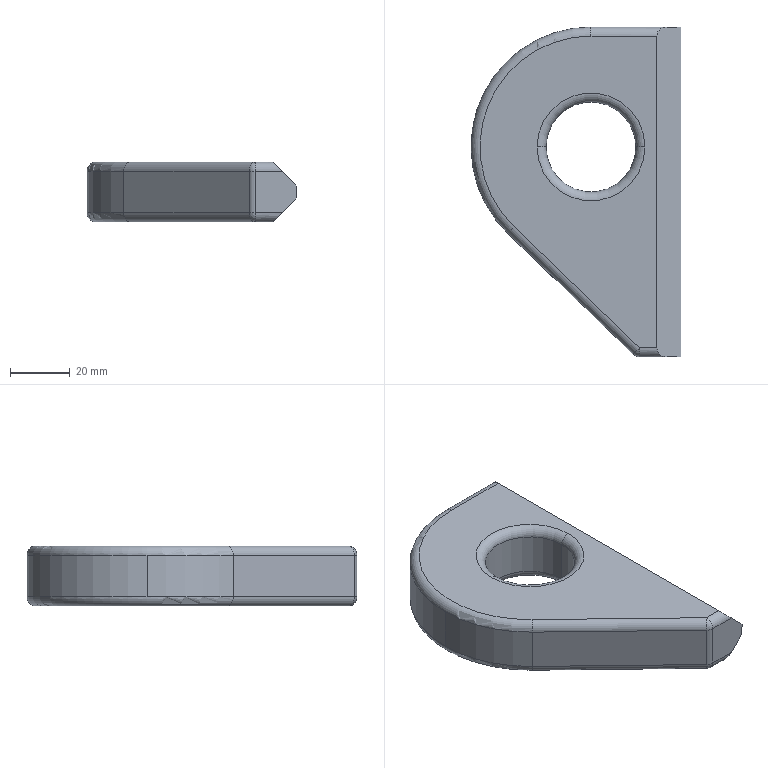Part | SolidWorks | features Fillet 3, Extrusion 1, ICE 1 | 1 solid | 27 faces | box 70 x 110 x 20 mm | volume 94979 mm3 | cylinder 11 | plane 8 | torus 6 | sphere 2 | commonest cylinder face diameters 6 x7 30 x2 80 x2
STEP:
#1=CARTESIAN_POINT('',(-15.,0.,3.));
#2=VERTEX_POINT('',#1);
#3=CARTESIAN_POINT('',(15.,0.,3.));
#4=VERTEX_POINT('',#3);
#5=CARTESIAN_POINT('',(0.,0.,3.));
#6=DIRECTION('',(0.,0.,-1.));
#7=DIRECTION('',(1.,0.,0.));
#8=AXIS2_PLACEMENT_3D('',#5,#6,#7);
#9=CIRCLE('',#8,15.);
#10=EDGE_CURVE('',#2,#4,#9,.T.);
#11=ORIENTED_EDGE('',*,*,#10,.F.);
#12=CARTESIAN_POINT('',(-18.,0.,0.));
#13=VERTEX_POINT('',#12);
#14=CARTESIAN_POINT('',(-18.,0.,3.));
#15=DIRECTION('',(0.,1.,0.));
#16=DIRECTION('',(0.,0.,1.));
#17=AXIS2_PLACEMENT_3D('',#14,#15,#16);
#18=CIRCLE('',#17,3.);
#19=EDGE_CURVE('',#2,#13,#18,.T.);
#20=ORIENTED_EDGE('',*,*,#19,.T.);
#21=CARTESIAN_POINT('',(18.,0.,0.));
#22=VERTEX_POINT('',#21);
#23=CARTESIAN_POINT('',(0.,0.,0.));
#24=DIRECTION('',(0.,0.,1.));
#25=DIRECTION('',(1.,0.,0.));
#26=AXIS2_PLACEMENT_3D('',#23,#24,#25);
#27=CIRCLE('',#26,18.);
#28=EDGE_CURVE('',#22,#13,#27,.T.);
#29=ORIENTED_EDGE('',*,*,#28,.F.);
#30=CARTESIAN_POINT('',(18.,0.,3.));
#31=DIRECTION('',(0.,-1.,0.));
#32=DIRECTION('',(0.,0.,-1.));
#33=AXIS2_PLACEMENT_3D('',#30,#31,#32);
#34=CIRCLE('',#33,3.);
#35=EDGE_CURVE('',#4,#22,#34,.T.);
#36=ORIENTED_EDGE('',*,*,#35,.F.);
#37=EDGE_LOOP('',(#11,#20,#29,#36));
#38=FACE_OUTER_BOUND('',#37,.T.);
#39=CARTESIAN_POINT('',(0.,0.,3.));
#40=DIRECTION('',(0.,0.,1.));
#41=DIRECTION('',(1.,0.,0.));
#42=AXIS2_PLACEMENT_3D('',#39,#40,#41);
#43=TOROIDAL_SURFACE('',#42,18.,3.);
#44=ADVANCED_FACE('',(#38),#43,.T.);
#45=CARTESIAN_POINT('',(-18.,0.,20.));
#46=VERTEX_POINT('',#45);
#47=CARTESIAN_POINT('',(18.,0.,20.));
#48=VERTEX_POINT('',#47);
#49=CARTESIAN_POINT('',(0.,0.,20.));
#50=DIRECTION('',(0.,0.,-1.));
#51=DIRECTION('',(1.,0.,0.));
#52=AXIS2_PLACEMENT_3D('',#49,#50,#51);
#53=CIRCLE('',#52,18.);
#54=EDGE_CURVE('',#46,#48,#53,.T.);
#55=ORIENTED_EDGE('',*,*,#54,.F.);
#56=CARTESIAN_POINT('',(-15.,0.,17.));
#57=VERTEX_POINT('',#56);
#58=CARTESIAN_POINT('',(-18.,0.,17.));
#59=DIRECTION('',(0.,1.,0.));
#60=DIRECTION('',(0.,0.,1.));
#61=AXIS2_PLACEMENT_3D('',#58,#59,#60);
#62=CIRCLE('',#61,3.);
#63=EDGE_CURVE('',#46,#57,#62,.T.);
#64=ORIENTED_EDGE('',*,*,#63,.T.);
#65=CARTESIAN_POINT('',(15.,0.,17.));
#66=VERTEX_POINT('',#65);
#67=CARTESIAN_POINT('',(0.,0.,17.));
#68=DIRECTION('',(0.,0.,1.));
#69=DIRECTION('',(1.,0.,0.));
#70=AXIS2_PLACEMENT_3D('',#67,#68,#69);
#71=CIRCLE('',#70,15.);
#72=EDGE_CURVE('',#66,#57,#71,.T.);
#73=ORIENTED_EDGE('',*,*,#72,.F.);
#74=CARTESIAN_POINT('',(18.,0.,17.));
#75=DIRECTION('',(0.,-1.,0.));
#76=DIRECTION('',(0.,0.,-1.));
#77=AXIS2_PLACEMENT_3D('',#74,#75,#76);
#78=CIRCLE('',#77,3.);
#79=EDGE_CURVE('',#48,#66,#78,.T.);
#80=ORIENTED_EDGE('',*,*,#79,.F.);
#81=EDGE_LOOP('',(#55,#64,#73,#80));
#82=FACE_OUTER_BOUND('',#81,.T.);
#83=CARTESIAN_POINT('',(0.,0.,17.));
#84=DIRECTION('',(0.,0.,1.));
#85=DIRECTION('',(1.,0.,0.));
#86=AXIS2_PLACEMENT_3D('',#83,#84,#85);
#87=TOROIDAL_SURFACE('',#86,18.,3.);
#88=ADVANCED_FACE('',(#82),#87,.T.);
#89=CARTESIAN_POINT('',(0.,0.,17.));
#90=DIRECTION('',(0.,0.,1.));
#91=DIRECTION('',(1.,0.,0.));
#92=AXIS2_PLACEMENT_3D('',#89,#90,#91);
#93=CIRCLE('',#92,15.);
#94=EDGE_CURVE('',#57,#66,#93,.T.);
#95=ORIENTED_EDGE('',*,*,#94,.T.);
#96=CARTESIAN_POINT('',(15.,0.,20.));
#97=DIRECTION('',(0.,0.,-1.));
#98=VECTOR('',#97,1000.);
#99=LINE('',#96,#98);
#100=EDGE_CURVE('',#66,#4,#99,.T.);
#101=ORIENTED_EDGE('',*,*,#100,.T.);
#102=CARTESIAN_POINT('',(0.,0.,3.));
#103=DIRECTION('',(0.,0.,-1.));
#104=DIRECTION('',(1.,0.,0.));
#105=AXIS2_PLACEMENT_3D('',#102,#103,#104);
#106=CIRCLE('',#105,15.);
#107=EDGE_CURVE('',#4,#2,#106,.T.);
#108=ORIENTED_EDGE('',*,*,#107,.T.);
#109=CARTESIAN_POINT('',(-15.,0.,20.));
#110=DIRECTION('',(0.,0.,-1.));
#111=VECTOR('',#110,1000.);
#112=LINE('',#109,#111);
#113=EDGE_CURVE('',#57,#2,#112,.T.);
#114=ORIENTED_EDGE('',*,*,#113,.F.);
#115=EDGE_LOOP('',(#95,#101,#108,#114));
#116=FACE_OUTER_BOUND('',#115,.T.);
#117=CARTESIAN_POINT('',(0.,0.,20.));
#118=DIRECTION('',(0.,0.,-1.));
#119=DIRECTION('',(-1.,0.,0.));
#120=AXIS2_PLACEMENT_3D('',#117,#118,#119);
#121=CYLINDRICAL_SURFACE('',#120,15.);
#122=ADVANCED_FACE('',(#116),#121,.F.);
#123=CARTESIAN_POINT('',(-27.754,-28.804,17.));
#124=VERTEX_POINT('',#123);
#125=CARTESIAN_POINT('',(-40.,0.,17.));
#126=VERTEX_POINT('',#125);
#127=CARTESIAN_POINT('',(0.,0.,17.));
#128=DIRECTION('',(0.,0.,-1.));
#129=DIRECTION('',(1.,0.,0.));
#130=AXIS2_PLACEMENT_3D('',#127,#128,#129);
#131=CIRCLE('',#130,40.);
#132=EDGE_CURVE('',#124,#126,#131,.T.);
#133=ORIENTED_EDGE('',*,*,#132,.T.);
#134=CARTESIAN_POINT('',(-40.,0.,3.));
#135=VERTEX_POINT('',#134);
#136=CARTESIAN_POINT('',(-40.,0.,20.));
#137=DIRECTION('',(0.,0.,-1.));
#138=VECTOR('',#137,1000.);
#139=LINE('',#136,#138);
#140=EDGE_CURVE('',#126,#135,#139,.T.);
#141=ORIENTED_EDGE('',*,*,#140,.T.);
#142=CARTESIAN_POINT('',(-27.754,-28.804,3.));
#143=VERTEX_POINT('',#142);
#144=CARTESIAN_POINT('',(0.,0.,3.));
#145=DIRECTION('',(0.,0.,1.));
#146=DIRECTION('',(1.,0.,0.));
#147=AXIS2_PLACEMENT_3D('',#144,#145,#146);
#148=CIRCLE('',#147,40.);
#149=EDGE_CURVE('',#135,#143,#148,.T.);
#150=ORIENTED_EDGE('',*,*,#149,.T.);
#151=CARTESIAN_POINT('',(-27.754,-28.804,20.));
#152=DIRECTION('',(0.,0.,-1.));
#153=VECTOR('',#152,1000.);
#154=LINE('',#151,#153);
#155=EDGE_CURVE('',#124,#143,#154,.T.);
#156=ORIENTED_EDGE('',*,*,#155,.F.);
#157=EDGE_LOOP('',(#133,#141,#150,#156));
#158=FACE_OUTER_BOUND('',#157,.T.);
#159=CARTESIAN_POINT('',(0.,0.,20.));
#160=DIRECTION('',(0.,0.,-1.));
#161=DIRECTION('',(-1.,0.,0.));
#162=AXIS2_PLACEMENT_3D('',#159,#160,#161);
#163=CYLINDRICAL_SURFACE('',#162,40.);
#164=ADVANCED_FACE('',(#158),#163,.T.);
#165=CARTESIAN_POINT('',(0.,0.,20.));
#166=DIRECTION('',(0.,0.,-1.));
#167=DIRECTION('',(1.,0.,0.));
#168=AXIS2_PLACEMENT_3D('',#165,#166,#167);
#169=CIRCLE('',#168,18.);
#170=EDGE_CURVE('',#48,#46,#169,.T.);
#171=ORIENTED_EDGE('',*,*,#170,.T.);
#172=ORIENTED_EDGE('',*,*,#54,.T.);
#173=EDGE_LOOP('',(#171,#172));
#174=FACE_BOUND('',#173,.T.);
#175=CARTESIAN_POINT('',(22.,-67.,20.));
#176=VERTEX_POINT('',#175);
#177=CARTESIAN_POINT('',(22.,37.,20.));
#178=VERTEX_POINT('',#177);
#179=CARTESIAN_POINT('',(22.,-70.,20.));
#180=DIRECTION('',(0.,1.,0.));
#181=VECTOR('',#180,1000.);
#182=LINE('',#179,#181);
#183=EDGE_CURVE('',#176,#178,#182,.T.);
#184=ORIENTED_EDGE('',*,*,#183,.T.);
#185=CARTESIAN_POINT('',(0.,37.,20.));
#186=VERTEX_POINT('',#185);
#187=CARTESIAN_POINT('',(0.,37.,20.));
#188=DIRECTION('',(-1.,0.,0.));
#189=VECTOR('',#188,1000.);
#190=LINE('',#187,#189);
#191=EDGE_CURVE('',#178,#186,#190,.T.);
#192=ORIENTED_EDGE('',*,*,#191,.T.);
#193=CARTESIAN_POINT('',(-25.673,-26.644,20.));
#194=VERTEX_POINT('',#193);
#195=CARTESIAN_POINT('',(0.,0.,20.));
#196=DIRECTION('',(0.,0.,1.));
#197=DIRECTION('',(1.,0.,0.));
#198=AXIS2_PLACEMENT_3D('',#195,#196,#197);
#199=CIRCLE('',#198,37.);
#200=EDGE_CURVE('',#186,#194,#199,.T.);
#201=ORIENTED_EDGE('',*,*,#200,.T.);
#202=CARTESIAN_POINT('',(16.21,-67.,20.));
#203=VERTEX_POINT('',#202);
#204=CARTESIAN_POINT('',(17.082,-67.84,20.));
#205=DIRECTION('',(0.7201,-0.6939,0.));
#206=VECTOR('',#205,1000.);
#207=LINE('',#204,#206);
#208=EDGE_CURVE('',#194,#203,#207,.T.);
#209=ORIENTED_EDGE('',*,*,#208,.T.);
#210=CARTESIAN_POINT('',(30.,-67.,20.));
#211=DIRECTION('',(1.,0.,0.));
#212=VECTOR('',#211,1000.);
#213=LINE('',#210,#212);
#214=EDGE_CURVE('',#203,#176,#213,.T.);
#215=ORIENTED_EDGE('',*,*,#214,.T.);
#216=EDGE_LOOP('',(#184,#192,#201,#209,#215));
#217=FACE_OUTER_BOUND('',#216,.T.);
#218=CARTESIAN_POINT('',(0.,0.,20.));
#219=DIRECTION('',(0.,0.,1.));
#220=DIRECTION('',(1.,0.,0.));
#221=AXIS2_PLACEMENT_3D('',#218,#219,#220);
#222=PLANE('',#221);
#223=ADVANCED_FACE('',(#174,#217),#222,.T.);
#224=ORIENTED_EDGE('',*,*,#28,.T.);
#225=CARTESIAN_POINT('',(0.,0.,0.));
#226=DIRECTION('',(0.,0.,1.));
#227=DIRECTION('',(1.,0.,0.));
#228=AXIS2_PLACEMENT_3D('',#225,#226,#227);
#229=CIRCLE('',#228,18.);
#230=EDGE_CURVE('',#13,#22,#229,.T.);
#231=ORIENTED_EDGE('',*,*,#230,.T.);
#232=EDGE_LOOP('',(#224,#231));
#233=FACE_BOUND('',#232,.T.);
#234=CARTESIAN_POINT('',(0.,37.,0.));
#235=VERTEX_POINT('',#234);
#236=CARTESIAN_POINT('',(22.,37.,0.));
#237=VERTEX_POINT('',#236);
#238=CARTESIAN_POINT('',(0.,37.,0.));
#239=DIRECTION('',(1.,0.,0.));
#240=VECTOR('',#239,1000.);
#241=LINE('',#238,#240);
#242=EDGE_CURVE('',#235,#237,#241,.T.);
#243=ORIENTED_EDGE('',*,*,#242,.T.);
#244=CARTESIAN_POINT('',(22.,-67.,0.));
#245=VERTEX_POINT('',#244);
#246=CARTESIAN_POINT('',(22.,-70.,0.));
#247=DIRECTION('',(0.,1.,0.));
#248=VECTOR('',#247,1000.);
#249=LINE('',#246,#248);
#250=EDGE_CURVE('',#245,#237,#249,.T.);
#251=ORIENTED_EDGE('',*,*,#250,.F.);
#252=CARTESIAN_POINT('',(16.21,-67.,0.));
#253=VERTEX_POINT('',#252);
#254=CARTESIAN_POINT('',(0.,-67.,0.));
#255=DIRECTION('',(-1.,0.,0.));
#256=VECTOR('',#255,1000.);
#257=LINE('',#254,#256);
#258=EDGE_CURVE('',#245,#253,#257,.T.);
#259=ORIENTED_EDGE('',*,*,#258,.T.);
#260=CARTESIAN_POINT('',(-25.673,-26.644,0.));
#261=VERTEX_POINT('',#260);
#262=CARTESIAN_POINT('',(-25.673,-26.644,0.));
#263=DIRECTION('',(-0.7201,0.6939,0.));
#264=VECTOR('',#263,1000.);
#265=LINE('',#262,#264);
#266=EDGE_CURVE('',#253,#261,#265,.T.);
#267=ORIENTED_EDGE('',*,*,#266,.T.);
#268=CARTESIAN_POINT('',(0.,0.,0.));
#269=DIRECTION('',(0.,0.,-1.));
#270=DIRECTION('',(1.,0.,0.));
#271=AXIS2_PLACEMENT_3D('',#268,#269,#270);
#272=CIRCLE('',#271,37.);
#273=EDGE_CURVE('',#261,#235,#272,.T.);
#274=ORIENTED_EDGE('',*,*,#273,.T.);
#275=EDGE_LOOP('',(#243,#251,#259,#267,#274));
#276=FACE_OUTER_BOUND('',#275,.T.);
#277=CARTESIAN_POINT('',(0.,0.,0.));
#278=DIRECTION('',(0.,0.,1.));
#279=DIRECTION('',(1.,0.,0.));
#280=AXIS2_PLACEMENT_3D('',#277,#278,#279);
#281=PLANE('',#280);
#282=ADVANCED_FACE('',(#233,#276),#281,.F.);
#283=ORIENTED_EDGE('',*,*,#140,.F.);
#284=CARTESIAN_POINT('',(0.,40.,17.));
#285=VERTEX_POINT('',#284);
#286=CARTESIAN_POINT('',(0.,0.,17.));
#287=DIRECTION('',(0.,0.,-1.));
#288=DIRECTION('',(1.,0.,0.));
#289=AXIS2_PLACEMENT_3D('',#286,#287,#288);
#290=CIRCLE('',#289,40.);
#291=EDGE_CURVE('',#126,#285,#290,.T.);
#292=ORIENTED_EDGE('',*,*,#291,.T.);
#293=CARTESIAN_POINT('',(0.,40.,3.));
#294=VERTEX_POINT('',#293);
#295=CARTESIAN_POINT('',(0.,40.,20.));
#296=DIRECTION('',(0.,0.,-1.));
#297=VECTOR('',#296,1000.);
#298=LINE('',#295,#297);
#299=EDGE_CURVE('',#285,#294,#298,.T.);
#300=ORIENTED_EDGE('',*,*,#299,.T.);
#301=CARTESIAN_POINT('',(0.,0.,3.));
#302=DIRECTION('',(0.,0.,1.));
#303=DIRECTION('',(1.,0.,0.));
#304=AXIS2_PLACEMENT_3D('',#301,#302,#303);
#305=CIRCLE('',#304,40.);
#306=EDGE_CURVE('',#294,#135,#305,.T.);
#307=ORIENTED_EDGE('',*,*,#306,.T.);
#308=EDGE_LOOP('',(#283,#292,#300,#307));
#309=FACE_OUTER_BOUND('',#308,.T.);
#310=CARTESIAN_POINT('',(0.,0.,20.));
#311=DIRECTION('',(0.,0.,-1.));
#312=DIRECTION('',(-1.,0.,0.));
#313=AXIS2_PLACEMENT_3D('',#310,#311,#312);
#314=CYLINDRICAL_SURFACE('',#313,40.);
#315=ADVANCED_FACE('',(#309),#314,.T.);
#316=CARTESIAN_POINT('',(14.129,-69.16,3.));
#317=VERTEX_POINT('',#316);
#318=CARTESIAN_POINT('',(-27.754,-28.804,3.));
#319=DIRECTION('',(0.7201,-0.6939,0.));
#320=VECTOR('',#319,1000.);
#321=LINE('',#318,#320);
#322=EDGE_CURVE('',#143,#317,#321,.T.);
#323=ORIENTED_EDGE('',*,*,#322,.T.);
#324=CARTESIAN_POINT('',(14.129,-69.16,17.));
#325=VERTEX_POINT('',#324);
#326=CARTESIAN_POINT('',(14.129,-69.16,20.));
#327=DIRECTION('',(0.,0.,1.));
#328=VECTOR('',#327,1000.);
#329=LINE('',#326,#328);
#330=EDGE_CURVE('',#317,#325,#329,.T.);
#331=ORIENTED_EDGE('',*,*,#330,.T.);
#332=CARTESIAN_POINT('',(-27.754,-28.804,17.));
#333=DIRECTION('',(-0.7201,0.6939,0.));
#334=VECTOR('',#333,1000.);
#335=LINE('',#332,#334);
#336=EDGE_CURVE('',#325,#124,#335,.T.);
#337=ORIENTED_EDGE('',*,*,#336,.T.);
#338=ORIENTED_EDGE('',*,*,#155,.T.);
#339=EDGE_LOOP('',(#323,#331,#337,#338));
#340=FACE_OUTER_BOUND('',#339,.T.);
#341=CARTESIAN_POINT('',(-27.754,-28.804,20.));
#342=DIRECTION('',(0.6939,0.7201,0.));
#343=DIRECTION('',(-0.7201,0.6939,0.));
#344=AXIS2_PLACEMENT_3D('',#341,#342,#343);
#345=PLANE('',#344);
#346=ADVANCED_FACE('',(#340),#345,.F.);
#347=CARTESIAN_POINT('',(30.,-70.,12.));
#348=VERTEX_POINT('',#347);
#349=CARTESIAN_POINT('',(30.,-70.,8.));
#350=VERTEX_POINT('',#349);
#351=CARTESIAN_POINT('',(30.,-70.,20.));
#352=DIRECTION('',(0.,0.,-1.));
#353=VECTOR('',#352,1000.);
#354=LINE('',#351,#353);
#355=EDGE_CURVE('',#348,#350,#354,.T.);
#356=ORIENTED_EDGE('',*,*,#355,.F.);
#357=CARTESIAN_POINT('',(25.,-70.,17.));
#358=VERTEX_POINT('',#357);
#359=CARTESIAN_POINT('',(30.,-70.,12.));
#360=DIRECTION('',(-0.7071,0.,0.7071));
#361=VECTOR('',#360,1000.);
#362=LINE('',#359,#361);
#363=EDGE_CURVE('',#348,#358,#362,.T.);
#364=ORIENTED_EDGE('',*,*,#363,.T.);
#365=CARTESIAN_POINT('',(16.21,-70.,17.));
#366=VERTEX_POINT('',#365);
#367=CARTESIAN_POINT('',(19.324,-70.,17.));
#368=DIRECTION('',(-1.,0.,0.));
#369=VECTOR('',#368,1000.);
#370=LINE('',#367,#369);
#371=EDGE_CURVE('',#358,#366,#370,.T.);
#372=ORIENTED_EDGE('',*,*,#371,.T.);
#373=CARTESIAN_POINT('',(16.21,-70.,3.));
#374=VERTEX_POINT('',#373);
#375=CARTESIAN_POINT('',(16.21,-70.,20.));
#376=DIRECTION('',(0.,0.,-1.));
#377=VECTOR('',#376,1000.);
#378=LINE('',#375,#377);
#379=EDGE_CURVE('',#366,#374,#378,.T.);
#380=ORIENTED_EDGE('',*,*,#379,.T.);
#381=CARTESIAN_POINT('',(25.,-70.,3.));
#382=VERTEX_POINT('',#381);
#383=CARTESIAN_POINT('',(15.,-70.,3.));
#384=DIRECTION('',(1.,0.,0.));
#385=VECTOR('',#384,1000.);
#386=LINE('',#383,#385);
#387=EDGE_CURVE('',#374,#382,#386,.T.);
#388=ORIENTED_EDGE('',*,*,#387,.T.);
#389=CARTESIAN_POINT('',(30.,-70.,8.));
#390=DIRECTION('',(0.7071,0.,0.7071));
#391=VECTOR('',#390,1000.);
#392=LINE('',#389,#391);
#393=EDGE_CURVE('',#382,#350,#392,.T.);
#394=ORIENTED_EDGE('',*,*,#393,.T.);
#395=EDGE_LOOP('',(#356,#364,#372,#380,#388,#394));
#396=FACE_OUTER_BOUND('',#395,.T.);
#397=CARTESIAN_POINT('',(15.,-70.,20.));
#398=DIRECTION('',(0.,1.,0.));
#399=DIRECTION('',(0.,0.,1.));
#400=AXIS2_PLACEMENT_3D('',#397,#398,#399);
#401=PLANE('',#400);
#402=ADVANCED_FACE('',(#396),#401,.F.);
#403=CARTESIAN_POINT('',(30.,40.,12.));
#404=VERTEX_POINT('',#403);
#405=CARTESIAN_POINT('',(30.,40.,8.));
#406=VERTEX_POINT('',#405);
#407=CARTESIAN_POINT('',(30.,40.,20.));
#408=DIRECTION('',(0.,0.,-1.));
#409=VECTOR('',#408,1000.);
#410=LINE('',#407,#409);
#411=EDGE_CURVE('',#404,#406,#410,.T.);
#412=ORIENTED_EDGE('',*,*,#411,.F.);
#413=CARTESIAN_POINT('',(30.,-70.,12.));
#414=DIRECTION('',(0.,1.,0.));
#415=VECTOR('',#414,1000.);
#416=LINE('',#413,#415);
#417=EDGE_CURVE('',#348,#404,#416,.T.);
#418=ORIENTED_EDGE('',*,*,#417,.F.);
#419=ORIENTED_EDGE('',*,*,#355,.T.);
#420=CARTESIAN_POINT('',(30.,-70.,8.));
#421=DIRECTION('',(0.,1.,0.));
#422=VECTOR('',#421,1000.);
#423=LINE('',#420,#422);
#424=EDGE_CURVE('',#350,#406,#423,.T.);
#425=ORIENTED_EDGE('',*,*,#424,.T.);
#426=EDGE_LOOP('',(#412,#418,#419,#425));
#427=FACE_OUTER_BOUND('',#426,.T.);
#428=CARTESIAN_POINT('',(30.,40.,20.));
#429=DIRECTION('',(-1.,0.,0.));
#430=DIRECTION('',(0.,-1.,0.));
#431=AXIS2_PLACEMENT_3D('',#428,#429,#430);
#432=PLANE('',#431);
#433=ADVANCED_FACE('',(#427),#432,.F.);
#434=CARTESIAN_POINT('',(25.,40.,17.));
#435=VERTEX_POINT('',#434);
#436=CARTESIAN_POINT('',(30.,40.,17.));
#437=DIRECTION('',(1.,0.,0.));
#438=VECTOR('',#437,1000.);
#439=LINE('',#436,#438);
#440=EDGE_CURVE('',#285,#435,#439,.T.);
#441=ORIENTED_EDGE('',*,*,#440,.T.);
#442=CARTESIAN_POINT('',(30.,40.,12.));
#443=DIRECTION('',(-0.7071,0.,0.7071));
#444=VECTOR('',#443,1000.);
#445=LINE('',#442,#444);
#446=EDGE_CURVE('',#404,#435,#445,.T.);
#447=ORIENTED_EDGE('',*,*,#446,.F.);
#448=ORIENTED_EDGE('',*,*,#411,.T.);
#449=CARTESIAN_POINT('',(25.,40.,3.));
#450=VERTEX_POINT('',#449);
#451=CARTESIAN_POINT('',(30.,40.,8.));
#452=DIRECTION('',(0.7071,0.,0.7071));
#453=VECTOR('',#452,1000.);
#454=LINE('',#451,#453);
#455=EDGE_CURVE('',#450,#406,#454,.T.);
#456=ORIENTED_EDGE('',*,*,#455,.F.);
#457=CARTESIAN_POINT('',(0.,40.,3.));
#458=DIRECTION('',(-1.,0.,0.));
#459=VECTOR('',#458,1000.);
#460=LINE('',#457,#459);
#461=EDGE_CURVE('',#450,#294,#460,.T.);
#462=ORIENTED_EDGE('',*,*,#461,.T.);
#463=ORIENTED_EDGE('',*,*,#299,.F.);
#464=EDGE_LOOP('',(#441,#447,#448,#456,#462,#463));
#465=FACE_OUTER_BOUND('',#464,.T.);
#466=CARTESIAN_POINT('',(0.,40.,20.));
#467=DIRECTION('',(0.,-1.,0.));
#468=DIRECTION('',(1.,0.,0.));
#469=AXIS2_PLACEMENT_3D('',#466,#467,#468);
#470=PLANE('',#469);
#471=ADVANCED_FACE('',(#465),#470,.F.);
#472=ORIENTED_EDGE('',*,*,#100,.F.);
#473=ORIENTED_EDGE('',*,*,#72,.T.);
#474=ORIENTED_EDGE('',*,*,#113,.T.);
#475=ORIENTED_EDGE('',*,*,#10,.T.);
#476=EDGE_LOOP('',(#472,#473,#474,#475));
#477=FACE_OUTER_BOUND('',#476,.T.);
#478=CARTESIAN_POINT('',(0.,0.,20.));
#479=DIRECTION('',(0.,0.,-1.));
#480=DIRECTION('',(-1.,0.,0.));
#481=AXIS2_PLACEMENT_3D('',#478,#479,#480);
#482=CYLINDRICAL_SURFACE('',#481,15.);
#483=ADVANCED_FACE('',(#477),#482,.F.);
#484=ORIENTED_EDGE('',*,*,#266,.F.);
#485=CARTESIAN_POINT('',(16.21,-67.,3.));
#486=DIRECTION('',(-0.7201,0.6939,0.));
#487=DIRECTION('',(0.6939,0.7201,0.));
#488=AXIS2_PLACEMENT_3D('',#485,#486,#487);
#489=CIRCLE('',#488,3.);
#490=EDGE_CURVE('',#253,#317,#489,.T.);
#491=ORIENTED_EDGE('',*,*,#490,.T.);
#492=ORIENTED_EDGE('',*,*,#322,.F.);
#493=CARTESIAN_POINT('',(-25.673,-26.644,3.));
#494=DIRECTION('',(-0.7201,0.6939,0.));
#495=DIRECTION('',(-0.6939,-0.7201,0.));
#496=AXIS2_PLACEMENT_3D('',#493,#494,#495);
#497=CIRCLE('',#496,3.);
#498=EDGE_CURVE('',#261,#143,#497,.T.);
#499=ORIENTED_EDGE('',*,*,#498,.F.);
#500=EDGE_LOOP('',(#484,#491,#492,#499));
#501=FACE_OUTER_BOUND('',#500,.T.);
#502=CARTESIAN_POINT('',(-25.673,-26.644,3.));
#503=DIRECTION('',(0.7201,-0.6939,0.));
#504=DIRECTION('',(0.6939,0.7201,0.));
#505=AXIS2_PLACEMENT_3D('',#502,#503,#504);
#506=CYLINDRICAL_SURFACE('',#505,3.);
#507=ADVANCED_FACE('',(#501),#506,.T.);
#508=ORIENTED_EDGE('',*,*,#498,.T.);
#509=ORIENTED_EDGE('',*,*,#149,.F.);
#510=ORIENTED_EDGE('',*,*,#306,.F.);
#511=CARTESIAN_POINT('',(0.,37.,3.));
#512=DIRECTION('',(1.,0.,0.));
#513=DIRECTION('',(0.,1.,0.));
#514=AXIS2_PLACEMENT_3D('',#511,#512,#513);
#515=CIRCLE('',#514,3.);
#516=EDGE_CURVE('',#235,#294,#515,.T.);
#517=ORIENTED_EDGE('',*,*,#516,.F.);
#518=ORIENTED_EDGE('',*,*,#273,.F.);
#519=EDGE_LOOP('',(#508,#509,#510,#517,#518));
#520=FACE_OUTER_BOUND('',#519,.T.);
#521=CARTESIAN_POINT('',(0.,0.,3.));
#522=DIRECTION('',(0.,0.,1.));
#523=DIRECTION('',(1.,0.,0.));
#524=AXIS2_PLACEMENT_3D('',#521,#522,#523);
#525=TOROIDAL_SURFACE('',#524,37.,3.);
#526=ADVANCED_FACE('',(#520),#525,.T.);
#527=CARTESIAN_POINT('',(22.,37.,0.));
#528=CARTESIAN_POINT('',(22.,38.757,0.));
#529=CARTESIAN_POINT('',(23.243,40.,1.243));
#530=CARTESIAN_POINT('',(25.,40.,3.));
#531=(BOUNDED_CURVE()B_SPLINE_CURVE(3,(#527,#528,#529,#530),.UNSPECIFIED.,.F.,.F.)B_SPLINE_CURVE_WITH_KNOTS((4,4),(0.,1.571),.UNSPECIFIED.)CURVE()GEOMETRIC_REPRESENTATION_ITEM()RATIONAL_B_SPLINE_CURVE((1.,0.8047,0.8047,1.))REPRESENTATION_ITEM(''));
#532=EDGE_CURVE('',#237,#450,#531,.T.);
#533=ORIENTED_EDGE('',*,*,#532,.F.);
#534=ORIENTED_EDGE('',*,*,#242,.F.);
#535=ORIENTED_EDGE('',*,*,#516,.T.);
#536=ORIENTED_EDGE('',*,*,#461,.F.);
#537=EDGE_LOOP('',(#533,#534,#535,#536));
#538=FACE_OUTER_BOUND('',#537,.T.);
#539=CARTESIAN_POINT('',(0.,37.,3.));
#540=DIRECTION('',(-1.,0.,0.));
#541=DIRECTION('',(0.,-1.,0.));
#542=AXIS2_PLACEMENT_3D('',#539,#540,#541);
#543=CYLINDRICAL_SURFACE('',#542,3.);
#544=ADVANCED_FACE('',(#538),#543,.T.);
#545=ORIENTED_EDGE('',*,*,#336,.F.);
#546=CARTESIAN_POINT('',(16.21,-67.,17.));
#547=DIRECTION('',(-0.7201,0.6939,0.));
#548=DIRECTION('',(-0.6939,-0.7201,0.));
#549=AXIS2_PLACEMENT_3D('',#546,#547,#548);
#550=CIRCLE('',#549,3.);
#551=EDGE_CURVE('',#325,#203,#550,.T.);
#552=ORIENTED_EDGE('',*,*,#551,.T.);
#553=ORIENTED_EDGE('',*,*,#208,.F.);
#554=CARTESIAN_POINT('',(-25.673,-26.644,17.));
#555=DIRECTION('',(-0.7201,0.6939,0.));
#556=DIRECTION('',(-0.6939,-0.7201,0.));
#557=AXIS2_PLACEMENT_3D('',#554,#555,#556);
#558=CIRCLE('',#557,3.);
#559=EDGE_CURVE('',#124,#194,#558,.T.);
#560=ORIENTED_EDGE('',*,*,#559,.F.);
#561=EDGE_LOOP('',(#545,#552,#553,#560));
#562=FACE_OUTER_BOUND('',#561,.T.);
#563=CARTESIAN_POINT('',(-25.673,-26.644,17.));
#564=DIRECTION('',(-0.7201,0.6939,0.));
#565=DIRECTION('',(-0.6939,-0.7201,0.));
#566=AXIS2_PLACEMENT_3D('',#563,#564,#565);
#567=CYLINDRICAL_SURFACE('',#566,3.);
#568=ADVANCED_FACE('',(#562),#567,.T.);
#569=ORIENTED_EDGE('',*,*,#559,.T.);
#570=ORIENTED_EDGE('',*,*,#200,.F.);
#571=CARTESIAN_POINT('',(0.,37.,17.));
#572=DIRECTION('',(1.,0.,0.));
#573=DIRECTION('',(0.,0.,-1.));
#574=AXIS2_PLACEMENT_3D('',#571,#572,#573);
#575=CIRCLE('',#574,3.);
#576=EDGE_CURVE('',#285,#186,#575,.T.);
#577=ORIENTED_EDGE('',*,*,#576,.F.);
#578=ORIENTED_EDGE('',*,*,#291,.F.);
#579=ORIENTED_EDGE('',*,*,#132,.F.);
#580=EDGE_LOOP('',(#569,#570,#577,#578,#579));
#581=FACE_OUTER_BOUND('',#580,.T.);
#582=CARTESIAN_POINT('',(0.,0.,17.));
#583=DIRECTION('',(0.,0.,1.));
#584=DIRECTION('',(1.,0.,0.));
#585=AXIS2_PLACEMENT_3D('',#582,#583,#584);
#586=TOROIDAL_SURFACE('',#585,37.,3.);
#587=ADVANCED_FACE('',(#581),#586,.T.);
#588=CARTESIAN_POINT('',(25.,40.,17.));
#589=CARTESIAN_POINT('',(23.243,40.,18.757));
#590=CARTESIAN_POINT('',(22.,38.757,20.));
#591=CARTESIAN_POINT('',(22.,37.,20.));
#592=(BOUNDED_CURVE()B_SPLINE_CURVE(3,(#588,#589,#590,#591),.UNSPECIFIED.,.F.,.F.)B_SPLINE_CURVE_WITH_KNOTS((4,4),(1.571,3.142),.UNSPECIFIED.)CURVE()GEOMETRIC_REPRESENTATION_ITEM()RATIONAL_B_SPLINE_CURVE((1.,0.8047,0.8047,1.))REPRESENTATION_ITEM(''));
#593=EDGE_CURVE('',#435,#178,#592,.T.);
#594=ORIENTED_EDGE('',*,*,#593,.F.);
#595=ORIENTED_EDGE('',*,*,#440,.F.);
#596=ORIENTED_EDGE('',*,*,#576,.T.);
#597=ORIENTED_EDGE('',*,*,#191,.F.);
#598=EDGE_LOOP('',(#594,#595,#596,#597));
#599=FACE_OUTER_BOUND('',#598,.T.);
#600=CARTESIAN_POINT('',(0.,37.,17.));
#601=DIRECTION('',(1.,0.,0.));
#602=DIRECTION('',(0.,1.,0.));
#603=AXIS2_PLACEMENT_3D('',#600,#601,#602);
#604=CYLINDRICAL_SURFACE('',#603,3.);
#605=ADVANCED_FACE('',(#599),#604,.T.);
#606=CARTESIAN_POINT('',(22.,-67.,20.));
#607=CARTESIAN_POINT('',(22.,-68.757,20.));
#608=CARTESIAN_POINT('',(23.243,-70.,18.757));
#609=CARTESIAN_POINT('',(25.,-70.,17.));
#610=(BOUNDED_CURVE()B_SPLINE_CURVE(3,(#606,#607,#608,#609),.UNSPECIFIED.,.F.,.F.)B_SPLINE_CURVE_WITH_KNOTS((4,4),(0.,1.571),.UNSPECIFIED.)CURVE()GEOMETRIC_REPRESENTATION_ITEM()RATIONAL_B_SPLINE_CURVE((1.,0.8047,0.8047,1.))REPRESENTATION_ITEM(''));
#611=EDGE_CURVE('',#176,#358,#610,.T.);
#612=ORIENTED_EDGE('',*,*,#611,.F.);
#613=ORIENTED_EDGE('',*,*,#214,.F.);
#614=CARTESIAN_POINT('',(16.21,-67.,17.));
#615=DIRECTION('',(-1.,0.,0.));
#616=DIRECTION('',(0.,0.,1.));
#617=AXIS2_PLACEMENT_3D('',#614,#615,#616);
#618=CIRCLE('',#617,3.);
#619=EDGE_CURVE('',#366,#203,#618,.T.);
#620=ORIENTED_EDGE('',*,*,#619,.F.);
#621=ORIENTED_EDGE('',*,*,#371,.F.);
#622=EDGE_LOOP('',(#612,#613,#620,#621));
#623=FACE_OUTER_BOUND('',#622,.T.);
#624=CARTESIAN_POINT('',(0.,-67.,17.));
#625=DIRECTION('',(-1.,0.,0.));
#626=DIRECTION('',(0.,0.,1.));
#627=AXIS2_PLACEMENT_3D('',#624,#625,#626);
#628=CYLINDRICAL_SURFACE('',#627,3.);
#629=ADVANCED_FACE('',(#623),#628,.T.);
#630=ORIENTED_EDGE('',*,*,#619,.T.);
#631=ORIENTED_EDGE('',*,*,#551,.F.);
#632=CARTESIAN_POINT('',(16.21,-67.,17.));
#633=DIRECTION('',(0.,0.,-1.));
#634=DIRECTION('',(-1.,0.,0.));
#635=AXIS2_PLACEMENT_3D('',#632,#633,#634);
#636=CIRCLE('',#635,3.);
#637=EDGE_CURVE('',#366,#325,#636,.T.);
#638=ORIENTED_EDGE('',*,*,#637,.F.);
#639=EDGE_LOOP('',(#630,#631,#638));
#640=FACE_OUTER_BOUND('',#639,.T.);
#641=CARTESIAN_POINT('',(16.21,-67.,17.));
#642=DIRECTION('',(0.,1.,0.));
#643=DIRECTION('',(1.,0.,0.));
#644=AXIS2_PLACEMENT_3D('',#641,#642,#643);
#645=SPHERICAL_SURFACE('',#644,3.);
#646=ADVANCED_FACE('',(#640),#645,.T.);
#647=ORIENTED_EDGE('',*,*,#637,.T.);
#648=ORIENTED_EDGE('',*,*,#330,.F.);
#649=CARTESIAN_POINT('',(16.21,-67.,3.));
#650=DIRECTION('',(0.,0.,-1.));
#651=DIRECTION('',(-1.,0.,0.));
#652=AXIS2_PLACEMENT_3D('',#649,#650,#651);
#653=CIRCLE('',#652,3.);
#654=EDGE_CURVE('',#374,#317,#653,.T.);
#655=ORIENTED_EDGE('',*,*,#654,.F.);
#656=ORIENTED_EDGE('',*,*,#379,.F.);
#657=EDGE_LOOP('',(#647,#648,#655,#656));
#658=FACE_OUTER_BOUND('',#657,.T.);
#659=CARTESIAN_POINT('',(16.21,-67.,20.));
#660=DIRECTION('',(0.,0.,-1.));
#661=DIRECTION('',(-1.,0.,0.));
#662=AXIS2_PLACEMENT_3D('',#659,#660,#661);
#663=CYLINDRICAL_SURFACE('',#662,3.);
#664=ADVANCED_FACE('',(#658),#663,.T.);
#665=ORIENTED_EDGE('',*,*,#654,.T.);
#666=ORIENTED_EDGE('',*,*,#490,.F.);
#667=CARTESIAN_POINT('',(16.21,-67.,3.));
#668=DIRECTION('',(1.,0.,0.));
#669=DIRECTION('',(0.,0.,-1.));
#670=AXIS2_PLACEMENT_3D('',#667,#668,#669);
#671=CIRCLE('',#670,3.);
#672=EDGE_CURVE('',#374,#253,#671,.T.);
#673=ORIENTED_EDGE('',*,*,#672,.F.);
#674=EDGE_LOOP('',(#665,#666,#673));
#675=FACE_OUTER_BOUND('',#674,.T.);
#676=CARTESIAN_POINT('',(16.21,-67.,3.));
#677=DIRECTION('',(0.,1.,0.));
#678=DIRECTION('',(1.,0.,0.));
#679=AXIS2_PLACEMENT_3D('',#676,#677,#678);
#680=SPHERICAL_SURFACE('',#679,3.);
#681=ADVANCED_FACE('',(#675),#680,.T.);
#682=CARTESIAN_POINT('',(25.,-70.,3.));
#683=CARTESIAN_POINT('',(23.243,-70.,1.243));
#684=CARTESIAN_POINT('',(22.,-68.757,0.));
#685=CARTESIAN_POINT('',(22.,-67.,0.));
#686=(BOUNDED_CURVE()B_SPLINE_CURVE(3,(#682,#683,#684,#685),.UNSPECIFIED.,.F.,.F.)B_SPLINE_CURVE_WITH_KNOTS((4,4),(1.571,3.142),.UNSPECIFIED.)CURVE()GEOMETRIC_REPRESENTATION_ITEM()RATIONAL_B_SPLINE_CURVE((1.,0.8047,0.8047,1.))REPRESENTATION_ITEM(''));
#687=EDGE_CURVE('',#382,#245,#686,.T.);
#688=ORIENTED_EDGE('',*,*,#687,.F.);
#689=ORIENTED_EDGE('',*,*,#387,.F.);
#690=ORIENTED_EDGE('',*,*,#672,.T.);
#691=ORIENTED_EDGE('',*,*,#258,.F.);
#692=EDGE_LOOP('',(#688,#689,#690,#691));
#693=FACE_OUTER_BOUND('',#692,.T.);
#694=CARTESIAN_POINT('',(15.,-67.,3.));
#695=DIRECTION('',(1.,0.,0.));
#696=DIRECTION('',(0.,0.,-1.));
#697=AXIS2_PLACEMENT_3D('',#694,#695,#696);
#698=CYLINDRICAL_SURFACE('',#697,3.);
#699=ADVANCED_FACE('',(#693),#698,.T.);
#700=ORIENTED_EDGE('',*,*,#532,.T.);
#701=ORIENTED_EDGE('',*,*,#455,.T.);
#702=ORIENTED_EDGE('',*,*,#424,.F.);
#703=ORIENTED_EDGE('',*,*,#393,.F.);
#704=ORIENTED_EDGE('',*,*,#687,.T.);
#705=ORIENTED_EDGE('',*,*,#250,.T.);
#706=EDGE_LOOP('',(#700,#701,#702,#703,#704,#705));
#707=FACE_OUTER_BOUND('',#706,.T.);
#708=CARTESIAN_POINT('',(30.,-70.,8.));
#709=DIRECTION('',(-0.7071,0.,0.7071));
#710=DIRECTION('',(0.7071,0.,0.7071));
#711=AXIS2_PLACEMENT_3D('',#708,#709,#710);
#712=PLANE('',#711);
#713=ADVANCED_FACE('',(#707),#712,.F.);
#714=ORIENTED_EDGE('',*,*,#593,.T.);
#715=ORIENTED_EDGE('',*,*,#183,.F.);
#716=ORIENTED_EDGE('',*,*,#611,.T.);
#717=ORIENTED_EDGE('',*,*,#363,.F.);
#718=ORIENTED_EDGE('',*,*,#417,.T.);
#719=ORIENTED_EDGE('',*,*,#446,.T.);
#720=EDGE_LOOP('',(#714,#715,#716,#717,#718,#719));
#721=FACE_OUTER_BOUND('',#720,.T.);
#722=CARTESIAN_POINT('',(30.,-70.,12.));
#723=DIRECTION('',(-0.7071,0.,-0.7071));
#724=DIRECTION('',(-0.7071,0.,0.7071));
#725=AXIS2_PLACEMENT_3D('',#722,#723,#724);
#726=PLANE('',#725);
#727=ADVANCED_FACE('',(#721),#726,.F.);
#728=ORIENTED_EDGE('',*,*,#63,.F.);
#729=ORIENTED_EDGE('',*,*,#170,.F.);
#730=ORIENTED_EDGE('',*,*,#79,.T.);
#731=ORIENTED_EDGE('',*,*,#94,.F.);
#732=EDGE_LOOP('',(#728,#729,#730,#731));
#733=FACE_OUTER_BOUND('',#732,.T.);
#734=CARTESIAN_POINT('',(0.,0.,17.));
#735=DIRECTION('',(0.,0.,1.));
#736=DIRECTION('',(1.,0.,0.));
#737=AXIS2_PLACEMENT_3D('',#734,#735,#736);
#738=TOROIDAL_SURFACE('',#737,18.,3.);
#739=ADVANCED_FACE('',(#733),#738,.T.);
#740=ORIENTED_EDGE('',*,*,#19,.F.);
#741=ORIENTED_EDGE('',*,*,#107,.F.);
#742=ORIENTED_EDGE('',*,*,#35,.T.);
#743=ORIENTED_EDGE('',*,*,#230,.F.);
#744=EDGE_LOOP('',(#740,#741,#742,#743));
#745=FACE_OUTER_BOUND('',#744,.T.);
#746=CARTESIAN_POINT('',(0.,0.,3.));
#747=DIRECTION('',(0.,0.,1.));
#748=DIRECTION('',(1.,0.,0.));
#749=AXIS2_PLACEMENT_3D('',#746,#747,#748);
#750=TOROIDAL_SURFACE('',#749,18.,3.);
#751=ADVANCED_FACE('',(#745),#750,.T.);
#752=CLOSED_SHELL('',(#44,#88,#122,#164,#223,#282,#315,#346,#402,#433,#471,#483,#507,#526,#544,#568,#587,#605,#629,#646,#664,#681,#699,#713,#727,#739,#751));
#753=MANIFOLD_SOLID_BREP('',#752);
#754=CARTESIAN_POINT('',(0.,0.,0.));
#755=DIRECTION('',(0.,0.,1.));
#756=DIRECTION('',(1.,0.,0.));
#757=AXIS2_PLACEMENT_3D('',#754,#755,#756);
#758=(LENGTH_UNIT()NAMED_UNIT(*)SI_UNIT(.MILLI.,.METRE.));
#759=UNCERTAINTY_MEASURE_WITH_UNIT(LENGTH_MEASURE(0.00001),#758,'','');
#760=(NAMED_UNIT(*)PLANE_ANGLE_UNIT()SI_UNIT($,.RADIAN.));
#761=(NAMED_UNIT(*)SI_UNIT($,.STERADIAN.)SOLID_ANGLE_UNIT());
#762=(GEOMETRIC_REPRESENTATION_CONTEXT(3)GLOBAL_UNCERTAINTY_ASSIGNED_CONTEXT((#759))GLOBAL_UNIT_ASSIGNED_CONTEXT((#758,#760,#761))REPRESENTATION_CONTEXT('',''));
#763=ADVANCED_BREP_SHAPE_REPRESENTATION('',(#753,#757),#762);